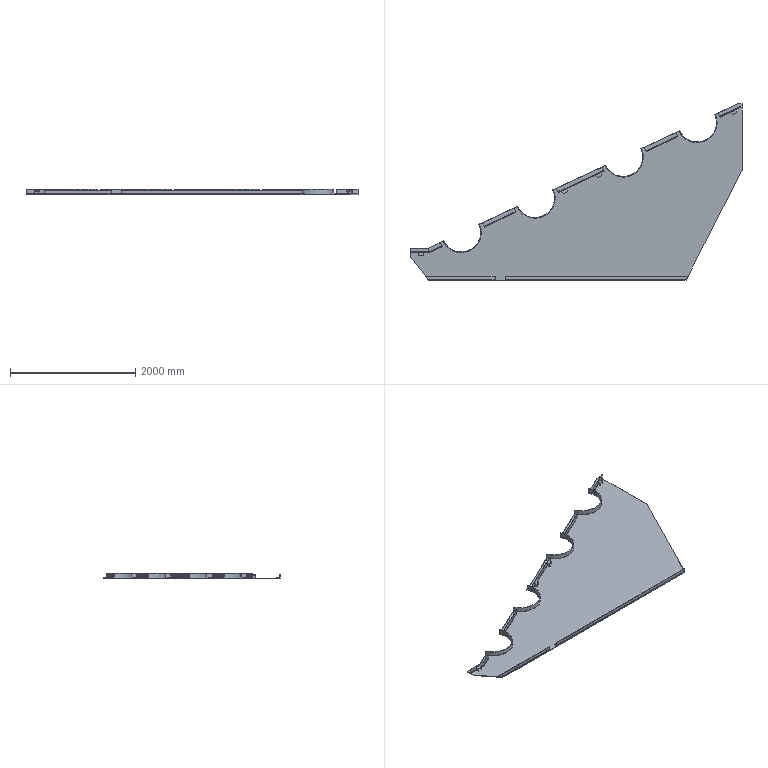Part | STEP file | Screen frame side plate assembly_Default<As machined> | 17 solids | 175 faces | box 5295 x 2809 x 83 mm | volume 63364081 mm3 | plane 135 | cylinder 40 | commonest cylinder face diameters 3.333 x16 618 x8 18 x6 628 x4 640 x4 14 x2